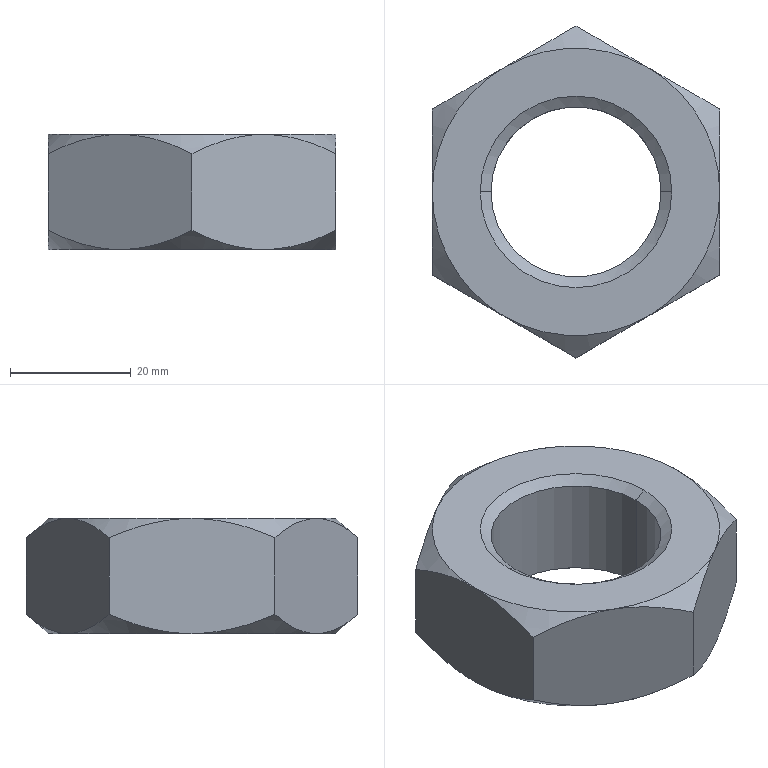Part | SolidWorks | features RevCut 4, Extrusion 1, LPattern 1 | 1 solid | 28 faces | box 47.625 x 54.993 x 19.075 mm | volume 25013 mm3 | cone 16 | plane 8 | cylinder 4 | commonest cylinder face diameters 28.179 x2 31.75 x2
STEP:
#1=CARTESIAN_POINT('',(-0.625,0.,-0.751));
#2=VERTEX_POINT('',#1);
#3=CARTESIAN_POINT('',(0.625,0.,-0.751));
#4=VERTEX_POINT('',#3);
#5=CARTESIAN_POINT('',(0.,0.,-0.751));
#6=DIRECTION('',(0.,0.,1.));
#7=DIRECTION('',(-1.,0.,0.));
#8=AXIS2_PLACEMENT_3D('',#5,#6,#7);
#9=CIRCLE('',#8,0.625);
#10=EDGE_CURVE('',#2,#4,#9,.T.);
#11=ORIENTED_EDGE('',*,*,#10,.F.);
#12=CARTESIAN_POINT('',(-0.625,0.,-0.75));
#13=VERTEX_POINT('',#12);
#14=CARTESIAN_POINT('',(-0.625,0.,-0.9857));
#15=DIRECTION('',(0.,0.,1.));
#16=VECTOR('',#15,39.37);
#17=LINE('',#14,#16);
#18=EDGE_CURVE('',#2,#13,#17,.T.);
#19=ORIENTED_EDGE('',*,*,#18,.T.);
#20=CARTESIAN_POINT('',(0.625,0.,-0.75));
#21=VERTEX_POINT('',#20);
#22=CARTESIAN_POINT('',(0.,0.,-0.75));
#23=DIRECTION('',(0.,0.,1.));
#24=DIRECTION('',(1.,0.,0.));
#25=AXIS2_PLACEMENT_3D('',#22,#23,#24);
#26=CIRCLE('',#25,0.625);
#27=EDGE_CURVE('',#13,#21,#26,.T.);
#28=ORIENTED_EDGE('',*,*,#27,.T.);
#29=CARTESIAN_POINT('',(0.625,0.,-0.9857));
#30=DIRECTION('',(0.,0.,1.));
#31=VECTOR('',#30,39.37);
#32=LINE('',#29,#31);
#33=EDGE_CURVE('',#4,#21,#32,.T.);
#34=ORIENTED_EDGE('',*,*,#33,.F.);
#35=EDGE_LOOP('',(#11,#19,#28,#34));
#36=FACE_OUTER_BOUND('',#35,.T.);
#37=CARTESIAN_POINT('',(0.,0.,-0.9857));
#38=DIRECTION('',(0.,0.,1.));
#39=DIRECTION('',(1.,0.,0.));
#40=AXIS2_PLACEMENT_3D('',#37,#38,#39);
#41=CYLINDRICAL_SURFACE('',#40,0.625);
#42=ADVANCED_FACE('',(#36),#41,.F.);
#43=CARTESIAN_POINT('',(-0.5547,0.,-0.7008));
#44=VERTEX_POINT('',#43);
#45=CARTESIAN_POINT('',(0.5547,0.,-0.7008));
#46=VERTEX_POINT('',#45);
#47=CARTESIAN_POINT('',(0.,0.,-0.7008));
#48=DIRECTION('',(0.,0.,1.));
#49=DIRECTION('',(-1.,0.,0.));
#50=AXIS2_PLACEMENT_3D('',#47,#48,#49);
#51=CIRCLE('',#50,0.5547);
#52=EDGE_CURVE('',#44,#46,#51,.T.);
#53=ORIENTED_EDGE('',*,*,#52,.T.);
#54=CARTESIAN_POINT('',(0.625,0.,-0.75));
#55=DIRECTION('',(0.8192,0.,-0.5736));
#56=VECTOR('',#55,39.37);
#57=LINE('',#54,#56);
#58=EDGE_CURVE('',#46,#21,#57,.T.);
#59=ORIENTED_EDGE('',*,*,#58,.T.);
#60=ORIENTED_EDGE('',*,*,#27,.F.);
#61=CARTESIAN_POINT('',(-0.625,0.,-0.75));
#62=DIRECTION('',(-0.8192,0.,-0.5736));
#63=VECTOR('',#62,39.37);
#64=LINE('',#61,#63);
#65=EDGE_CURVE('',#44,#13,#64,.T.);
#66=ORIENTED_EDGE('',*,*,#65,.F.);
#67=EDGE_LOOP('',(#53,#59,#60,#66));
#68=FACE_OUTER_BOUND('',#67,.T.);
#69=CARTESIAN_POINT('',(0.,0.,-0.75));
#70=DIRECTION('',(0.,0.,-1.));
#71=DIRECTION('',(-1.,0.,0.));
#72=AXIS2_PLACEMENT_3D('',#69,#70,#71);
#73=CONICAL_SURFACE('',#72,0.625,0.9599);
#74=ADVANCED_FACE('',(#68),#73,.F.);
#75=CARTESIAN_POINT('',(0.5547,0.,-0.04922));
#76=VERTEX_POINT('',#75);
#77=CARTESIAN_POINT('',(-0.5547,0.,-0.04922));
#78=VERTEX_POINT('',#77);
#79=CARTESIAN_POINT('',(0.,0.,-0.04922));
#80=DIRECTION('',(0.,0.,-1.));
#81=DIRECTION('',(1.,0.,0.));
#82=AXIS2_PLACEMENT_3D('',#79,#80,#81);
#83=CIRCLE('',#82,0.5547);
#84=EDGE_CURVE('',#76,#78,#83,.T.);
#85=ORIENTED_EDGE('',*,*,#84,.T.);
#86=CARTESIAN_POINT('',(-0.625,0.,0.));
#87=VERTEX_POINT('',#86);
#88=CARTESIAN_POINT('',(-0.5477,0.,-0.05415));
#89=DIRECTION('',(-0.8192,0.,0.5736));
#90=VECTOR('',#89,39.37);
#91=LINE('',#88,#90);
#92=EDGE_CURVE('',#78,#87,#91,.T.);
#93=ORIENTED_EDGE('',*,*,#92,.T.);
#94=CARTESIAN_POINT('',(0.625,0.,0.));
#95=VERTEX_POINT('',#94);
#96=CARTESIAN_POINT('',(0.,0.,0.));
#97=DIRECTION('',(0.,0.,1.));
#98=DIRECTION('',(1.,0.,0.));
#99=AXIS2_PLACEMENT_3D('',#96,#97,#98);
#100=CIRCLE('',#99,0.625);
#101=EDGE_CURVE('',#87,#95,#100,.T.);
#102=ORIENTED_EDGE('',*,*,#101,.T.);
#103=CARTESIAN_POINT('',(0.5477,0.,-0.05415));
#104=DIRECTION('',(0.8192,0.,0.5736));
#105=VECTOR('',#104,39.37);
#106=LINE('',#103,#105);
#107=EDGE_CURVE('',#76,#95,#106,.T.);
#108=ORIENTED_EDGE('',*,*,#107,.F.);
#109=EDGE_LOOP('',(#85,#93,#102,#108));
#110=FACE_OUTER_BOUND('',#109,.T.);
#111=CARTESIAN_POINT('',(0.,0.,-0.05415));
#112=DIRECTION('',(0.,0.,1.));
#113=DIRECTION('',(1.,0.,0.));
#114=AXIS2_PLACEMENT_3D('',#111,#112,#113);
#115=CONICAL_SURFACE('',#114,0.5477,0.9599);
#116=ADVANCED_FACE('',(#110),#115,.F.);
#117=ORIENTED_EDGE('',*,*,#52,.F.);
#118=CARTESIAN_POINT('',(-0.5547,0.,-0.751));
#119=DIRECTION('',(0.,0.,1.));
#120=VECTOR('',#119,39.37);
#121=LINE('',#118,#120);
#122=EDGE_CURVE('',#44,#78,#121,.T.);
#123=ORIENTED_EDGE('',*,*,#122,.T.);
#124=ORIENTED_EDGE('',*,*,#84,.F.);
#125=CARTESIAN_POINT('',(0.5547,0.,-0.751));
#126=DIRECTION('',(0.,0.,1.));
#127=VECTOR('',#126,39.37);
#128=LINE('',#125,#127);
#129=EDGE_CURVE('',#46,#76,#128,.T.);
#130=ORIENTED_EDGE('',*,*,#129,.F.);
#131=EDGE_LOOP('',(#117,#123,#124,#130));
#132=FACE_OUTER_BOUND('',#131,.T.);
#133=CARTESIAN_POINT('',(0.,0.,-0.751));
#134=DIRECTION('',(0.,0.,1.));
#135=DIRECTION('',(1.,0.,0.));
#136=AXIS2_PLACEMENT_3D('',#133,#134,#135);
#137=CYLINDRICAL_SURFACE('',#136,0.5547);
#138=ADVANCED_FACE('',(#132),#137,.F.);
#139=ORIENTED_EDGE('',*,*,#122,.F.);
#140=CARTESIAN_POINT('',(0.,0.,-0.7008));
#141=DIRECTION('',(0.,0.,1.));
#142=DIRECTION('',(-1.,0.,0.));
#143=AXIS2_PLACEMENT_3D('',#140,#141,#142);
#144=CIRCLE('',#143,0.5547);
#145=EDGE_CURVE('',#46,#44,#144,.T.);
#146=ORIENTED_EDGE('',*,*,#145,.F.);
#147=ORIENTED_EDGE('',*,*,#129,.T.);
#148=CARTESIAN_POINT('',(0.,0.,-0.04922));
#149=DIRECTION('',(0.,0.,-1.));
#150=DIRECTION('',(1.,0.,0.));
#151=AXIS2_PLACEMENT_3D('',#148,#149,#150);
#152=CIRCLE('',#151,0.5547);
#153=EDGE_CURVE('',#78,#76,#152,.T.);
#154=ORIENTED_EDGE('',*,*,#153,.F.);
#155=EDGE_LOOP('',(#139,#146,#147,#154));
#156=FACE_OUTER_BOUND('',#155,.T.);
#157=CARTESIAN_POINT('',(0.,0.,-0.751));
#158=DIRECTION('',(0.,0.,1.));
#159=DIRECTION('',(1.,0.,0.));
#160=AXIS2_PLACEMENT_3D('',#157,#158,#159);
#161=CYLINDRICAL_SURFACE('',#160,0.5547);
#162=ADVANCED_FACE('',(#156),#161,.F.);
#163=CARTESIAN_POINT('',(-0.9375,0.5413,-0.626));
#164=VERTEX_POINT('',#163);
#165=CARTESIAN_POINT('',(-0.9375,0.5413,-0.125));
#166=VERTEX_POINT('',#165);
#167=CARTESIAN_POINT('',(-0.9375,0.5413,-0.751));
#168=DIRECTION('',(0.,0.,1.));
#169=VECTOR('',#168,39.37);
#170=LINE('',#167,#169);
#171=EDGE_CURVE('',#164,#166,#170,.T.);
#172=ORIENTED_EDGE('',*,*,#171,.T.);
#173=CARTESIAN_POINT('',(-0.4688,0.8119,0.));
#174=VERTEX_POINT('',#173);
#175=CARTESIAN_POINT('',(-0.9375,0.5413,-0.125));
#176=CARTESIAN_POINT('',(-0.8627,0.5845,-0.08778));
#177=CARTESIAN_POINT('',(-0.7867,0.6283,-0.05655));
#178=CARTESIAN_POINT('',(-0.6698,0.6958,-0.02358));
#179=CARTESIAN_POINT('',(-0.6304,0.7186,-0.01492));
#180=CARTESIAN_POINT('',(-0.5704,0.7532,-0.006076));
#181=CARTESIAN_POINT('',(-0.5503,0.7648,-0.003818));
#182=CARTESIAN_POINT('',(-0.5098,0.7882,-0.0007797));
#183=CARTESIAN_POINT('',(-0.4893,0.8,0.));
#184=CARTESIAN_POINT('',(-0.4688,0.8119,0.));
#185=B_SPLINE_CURVE_WITH_KNOTS('',3,(#175,#176,#177,#178,#179,#180,#181,#182,#183,#184),.UNSPECIFIED.,.F.,.F.,(4,2,2,2,4),(0.000000248,0.007055,0.01058,0.01235,0.01411),.UNSPECIFIED.);
#186=EDGE_CURVE('',#166,#174,#185,.T.);
#187=ORIENTED_EDGE('',*,*,#186,.T.);
#188=CARTESIAN_POINT('',(0.,1.083,-0.125));
#189=VERTEX_POINT('',#188);
#190=CARTESIAN_POINT('',(-0.4688,0.8119,0.));
#191=CARTESIAN_POINT('',(-0.3871,0.8591,0.));
#192=CARTESIAN_POINT('',(-0.3075,0.905,-0.01242));
#193=CARTESIAN_POINT('',(-0.1905,0.9726,-0.04534));
#194=CARTESIAN_POINT('',(-0.1518,0.9949,-0.05867));
#195=CARTESIAN_POINT('',(-0.07528,1.039,-0.08921));
#196=CARTESIAN_POINT('',(-0.03734,1.061,-0.1064));
#197=CARTESIAN_POINT('',(0.,1.083,-0.125));
#198=B_SPLINE_CURVE_WITH_KNOTS('',3,(#190,#191,#192,#193,#194,#195,#196,#197),.UNSPECIFIED.,.F.,.F.,(4,2,2,4),(0.01411,0.02113,0.02464,0.02815),.UNSPECIFIED.);
#199=EDGE_CURVE('',#174,#189,#198,.T.);
#200=ORIENTED_EDGE('',*,*,#199,.T.);
#201=CARTESIAN_POINT('',(0.,1.083,-0.626));
#202=VERTEX_POINT('',#201);
#203=CARTESIAN_POINT('',(0.,1.083,-0.751));
#204=DIRECTION('',(0.,0.,1.));
#205=VECTOR('',#204,39.37);
#206=LINE('',#203,#205);
#207=EDGE_CURVE('',#202,#189,#206,.T.);
#208=ORIENTED_EDGE('',*,*,#207,.F.);
#209=CARTESIAN_POINT('',(-0.4688,0.8119,-0.751));
#210=VERTEX_POINT('',#209);
#211=CARTESIAN_POINT('',(-0.4688,0.8119,-0.751));
#212=CARTESIAN_POINT('',(-0.3871,0.8591,-0.751));
#213=CARTESIAN_POINT('',(-0.3075,0.905,-0.7386));
#214=CARTESIAN_POINT('',(-0.1905,0.9726,-0.7057));
#215=CARTESIAN_POINT('',(-0.1518,0.9949,-0.6923));
#216=CARTESIAN_POINT('',(-0.07528,1.039,-0.6618));
#217=CARTESIAN_POINT('',(-0.03734,1.061,-0.6446));
#218=CARTESIAN_POINT('',(0.,1.083,-0.626));
#219=B_SPLINE_CURVE_WITH_KNOTS('',3,(#211,#212,#213,#214,#215,#216,#217,#218),.UNSPECIFIED.,.F.,.F.,(4,2,2,4),(0.01411,0.02113,0.02464,0.02815),.UNSPECIFIED.);
#220=EDGE_CURVE('',#210,#202,#219,.T.);
#221=ORIENTED_EDGE('',*,*,#220,.F.);
#222=CARTESIAN_POINT('',(-0.9375,0.5413,-0.626));
#223=CARTESIAN_POINT('',(-0.8627,0.5845,-0.6632));
#224=CARTESIAN_POINT('',(-0.7867,0.6283,-0.6944));
#225=CARTESIAN_POINT('',(-0.6698,0.6958,-0.7274));
#226=CARTESIAN_POINT('',(-0.6304,0.7186,-0.7361));
#227=CARTESIAN_POINT('',(-0.5704,0.7532,-0.7449));
#228=CARTESIAN_POINT('',(-0.5503,0.7648,-0.7472));
#229=CARTESIAN_POINT('',(-0.5098,0.7882,-0.7502));
#230=CARTESIAN_POINT('',(-0.4893,0.8,-0.751));
#231=CARTESIAN_POINT('',(-0.4688,0.8119,-0.751));
#232=B_SPLINE_CURVE_WITH_KNOTS('',3,(#222,#223,#224,#225,#226,#227,#228,#229,#230,#231),.UNSPECIFIED.,.F.,.F.,(4,2,2,2,4),(0.000000248,0.007055,0.01058,0.01235,0.01411),.UNSPECIFIED.);
#233=EDGE_CURVE('',#164,#210,#232,.T.);
#234=ORIENTED_EDGE('',*,*,#233,.F.);
#235=EDGE_LOOP('',(#172,#187,#200,#208,#221,#234));
#236=FACE_OUTER_BOUND('',#235,.T.);
#237=CARTESIAN_POINT('',(0.,1.083,-0.751));
#238=DIRECTION('',(-0.5,0.866,0.));
#239=DIRECTION('',(-0.866,-0.5,0.));
#240=AXIS2_PLACEMENT_3D('',#237,#238,#239);
#241=PLANE('',#240);
#242=ADVANCED_FACE('',(#236),#241,.T.);
#243=ORIENTED_EDGE('',*,*,#207,.T.);
#244=CARTESIAN_POINT('',(0.4688,0.8119,0.));
#245=VERTEX_POINT('',#244);
#246=CARTESIAN_POINT('',(0.,1.083,-0.125));
#247=CARTESIAN_POINT('',(0.0748,1.039,-0.08778));
#248=CARTESIAN_POINT('',(0.1508,0.9955,-0.05655));
#249=CARTESIAN_POINT('',(0.2677,0.928,-0.02358));
#250=CARTESIAN_POINT('',(0.3071,0.9052,-0.01492));
#251=CARTESIAN_POINT('',(0.3671,0.8706,-0.006076));
#252=CARTESIAN_POINT('',(0.3872,0.859,-0.003818));
#253=CARTESIAN_POINT('',(0.4277,0.8356,-0.0007797));
#254=CARTESIAN_POINT('',(0.4482,0.8237,0.));
#255=CARTESIAN_POINT('',(0.4688,0.8119,0.));
#256=B_SPLINE_CURVE_WITH_KNOTS('',3,(#246,#247,#248,#249,#250,#251,#252,#253,#254,#255),.UNSPECIFIED.,.F.,.F.,(4,2,2,2,4),(0.000000248,0.007055,0.01058,0.01235,0.01411),.UNSPECIFIED.);
#257=EDGE_CURVE('',#189,#245,#256,.T.);
#258=ORIENTED_EDGE('',*,*,#257,.T.);
#259=CARTESIAN_POINT('',(0.9375,0.5413,-0.125));
#260=VERTEX_POINT('',#259);
#261=CARTESIAN_POINT('',(0.4688,0.8119,0.));
#262=CARTESIAN_POINT('',(0.5504,0.7647,0.));
#263=CARTESIAN_POINT('',(0.63,0.7188,-0.01242));
#264=CARTESIAN_POINT('',(0.747,0.6512,-0.04534));
#265=CARTESIAN_POINT('',(0.7857,0.6289,-0.05867));
#266=CARTESIAN_POINT('',(0.8622,0.5847,-0.08921));
#267=CARTESIAN_POINT('',(0.9002,0.5628,-0.1064));
#268=CARTESIAN_POINT('',(0.9375,0.5413,-0.125));
#269=B_SPLINE_CURVE_WITH_KNOTS('',3,(#261,#262,#263,#264,#265,#266,#267,#268),.UNSPECIFIED.,.F.,.F.,(4,2,2,4),(0.01411,0.02113,0.02464,0.02815),.UNSPECIFIED.);
#270=EDGE_CURVE('',#245,#260,#269,.T.);
#271=ORIENTED_EDGE('',*,*,#270,.T.);
#272=CARTESIAN_POINT('',(0.9375,0.5413,-0.626));
#273=VERTEX_POINT('',#272);
#274=CARTESIAN_POINT('',(0.9375,0.5413,-0.751));
#275=DIRECTION('',(0.,0.,1.));
#276=VECTOR('',#275,39.37);
#277=LINE('',#274,#276);
#278=EDGE_CURVE('',#273,#260,#277,.T.);
#279=ORIENTED_EDGE('',*,*,#278,.F.);
#280=CARTESIAN_POINT('',(0.4688,0.8119,-0.751));
#281=VERTEX_POINT('',#280);
#282=CARTESIAN_POINT('',(0.4688,0.8119,-0.751));
#283=CARTESIAN_POINT('',(0.5504,0.7647,-0.751));
#284=CARTESIAN_POINT('',(0.63,0.7188,-0.7386));
#285=CARTESIAN_POINT('',(0.747,0.6512,-0.7057));
#286=CARTESIAN_POINT('',(0.7857,0.6289,-0.6923));
#287=CARTESIAN_POINT('',(0.8622,0.5847,-0.6618));
#288=CARTESIAN_POINT('',(0.9002,0.5628,-0.6446));
#289=CARTESIAN_POINT('',(0.9375,0.5413,-0.626));
#290=B_SPLINE_CURVE_WITH_KNOTS('',3,(#282,#283,#284,#285,#286,#287,#288,#289),.UNSPECIFIED.,.F.,.F.,(4,2,2,4),(0.01411,0.02113,0.02464,0.02815),.UNSPECIFIED.);
#291=EDGE_CURVE('',#281,#273,#290,.T.);
#292=ORIENTED_EDGE('',*,*,#291,.F.);
#293=CARTESIAN_POINT('',(0.,1.083,-0.626));
#294=CARTESIAN_POINT('',(0.0748,1.039,-0.6632));
#295=CARTESIAN_POINT('',(0.1508,0.9955,-0.6944));
#296=CARTESIAN_POINT('',(0.2677,0.928,-0.7274));
#297=CARTESIAN_POINT('',(0.3071,0.9052,-0.7361));
#298=CARTESIAN_POINT('',(0.3671,0.8706,-0.7449));
#299=CARTESIAN_POINT('',(0.3872,0.859,-0.7472));
#300=CARTESIAN_POINT('',(0.4277,0.8356,-0.7502));
#301=CARTESIAN_POINT('',(0.4482,0.8237,-0.751));
#302=CARTESIAN_POINT('',(0.4688,0.8119,-0.751));
#303=B_SPLINE_CURVE_WITH_KNOTS('',3,(#293,#294,#295,#296,#297,#298,#299,#300,#301,#302),.UNSPECIFIED.,.F.,.F.,(4,2,2,2,4),(0.000000248,0.007055,0.01058,0.01235,0.01411),.UNSPECIFIED.);
#304=EDGE_CURVE('',#202,#281,#303,.T.);
#305=ORIENTED_EDGE('',*,*,#304,.F.);
#306=EDGE_LOOP('',(#243,#258,#271,#279,#292,#305));
#307=FACE_OUTER_BOUND('',#306,.T.);
#308=CARTESIAN_POINT('',(0.9375,0.5413,-0.751));
#309=DIRECTION('',(0.5,0.866,0.));
#310=DIRECTION('',(-0.866,0.5,0.));
#311=AXIS2_PLACEMENT_3D('',#308,#309,#310);
#312=PLANE('',#311);
#313=ADVANCED_FACE('',(#307),#312,.T.);
#314=CARTESIAN_POINT('',(0.9375,-0.5413,-0.125));
#315=VERTEX_POINT('',#314);
#316=CARTESIAN_POINT('',(0.9375,0.,0.));
#317=VERTEX_POINT('',#316);
#318=CARTESIAN_POINT('',(0.9375,-0.5413,-0.125));
#319=CARTESIAN_POINT('',(0.9375,-0.4985,-0.1066));
#320=CARTESIAN_POINT('',(0.9375,-0.4551,-0.08948));
#321=CARTESIAN_POINT('',(0.9375,-0.3663,-0.05876));
#322=CARTESIAN_POINT('',(0.9375,-0.3214,-0.04534));
#323=CARTESIAN_POINT('',(0.9375,-0.1858,-0.01233));
#324=CARTESIAN_POINT('',(0.9375,-0.09391,0.));
#325=CARTESIAN_POINT('',(0.9375,0.,0.));
#326=B_SPLINE_CURVE_WITH_KNOTS('',3,(#318,#319,#320,#321,#322,#323,#324,#325),.UNSPECIFIED.,.F.,.F.,(4,2,2,4),(0.01925,0.02278,0.02631,0.03337),.UNSPECIFIED.);
#327=EDGE_CURVE('',#315,#317,#326,.T.);
#328=ORIENTED_EDGE('',*,*,#327,.F.);
#329=CARTESIAN_POINT('',(0.9375,-0.5413,-0.626));
#330=VERTEX_POINT('',#329);
#331=CARTESIAN_POINT('',(0.9375,-0.5413,-0.751));
#332=DIRECTION('',(0.,0.,1.));
#333=VECTOR('',#332,39.37);
#334=LINE('',#331,#333);
#335=EDGE_CURVE('',#330,#315,#334,.T.);
#336=ORIENTED_EDGE('',*,*,#335,.F.);
#337=CARTESIAN_POINT('',(0.9375,0.,-0.751));
#338=VERTEX_POINT('',#337);
#339=CARTESIAN_POINT('',(0.9375,-0.5413,-0.626));
#340=CARTESIAN_POINT('',(0.9375,-0.4985,-0.6444));
#341=CARTESIAN_POINT('',(0.9375,-0.4551,-0.6615));
#342=CARTESIAN_POINT('',(0.9375,-0.3663,-0.6922));
#343=CARTESIAN_POINT('',(0.9375,-0.3214,-0.7057));
#344=CARTESIAN_POINT('',(0.9375,-0.1858,-0.7387));
#345=CARTESIAN_POINT('',(0.9375,-0.09391,-0.751));
#346=CARTESIAN_POINT('',(0.9375,0.,-0.751));
#347=B_SPLINE_CURVE_WITH_KNOTS('',3,(#339,#340,#341,#342,#343,#344,#345,#346),.UNSPECIFIED.,.F.,.F.,(4,2,2,4),(0.01925,0.02278,0.02631,0.03337),.UNSPECIFIED.);
#348=EDGE_CURVE('',#330,#338,#347,.T.);
#349=ORIENTED_EDGE('',*,*,#348,.T.);
#350=CARTESIAN_POINT('',(0.9375,0.,-0.751));
#351=CARTESIAN_POINT('',(0.9375,0.0234,-0.751));
#352=CARTESIAN_POINT('',(0.9375,0.047,-0.7502));
#353=CARTESIAN_POINT('',(0.9375,0.09377,-0.7472));
#354=CARTESIAN_POINT('',(0.9375,0.117,-0.745));
#355=CARTESIAN_POINT('',(0.9375,0.1862,-0.7362));
#356=CARTESIAN_POINT('',(0.9375,0.2318,-0.7275));
#357=CARTESIAN_POINT('',(0.9375,0.322,-0.7055));
#358=CARTESIAN_POINT('',(0.9375,0.3666,-0.6921));
#359=CARTESIAN_POINT('',(0.9375,0.4329,-0.6692));
#360=CARTESIAN_POINT('',(0.9375,0.4549,-0.6611));
#361=CARTESIAN_POINT('',(0.9375,0.4984,-0.6441));
#362=CARTESIAN_POINT('',(0.9375,0.5199,-0.6352));
#363=CARTESIAN_POINT('',(0.9375,0.5413,-0.626));
#364=B_SPLINE_CURVE_WITH_KNOTS('',3,(#350,#351,#352,#353,#354,#355,#356,#357,#358,#359,#360,#361,#362,#363),.UNSPECIFIED.,.F.,.F.,(4,2,2,2,2,2,4),(0.03337,0.03513,0.03689,0.04041,0.04394,0.0457,0.04746),.UNSPECIFIED.);
#365=EDGE_CURVE('',#338,#273,#364,.T.);
#366=ORIENTED_EDGE('',*,*,#365,.T.);
#367=ORIENTED_EDGE('',*,*,#278,.T.);
#368=CARTESIAN_POINT('',(0.9375,0.,0.));
#369=CARTESIAN_POINT('',(0.9375,0.0234,0.));
#370=CARTESIAN_POINT('',(0.9375,0.047,-0.0007652));
#371=CARTESIAN_POINT('',(0.9375,0.09377,-0.003783));
#372=CARTESIAN_POINT('',(0.9375,0.117,-0.00603));
#373=CARTESIAN_POINT('',(0.9375,0.1862,-0.01485));
#374=CARTESIAN_POINT('',(0.9375,0.2318,-0.0235));
#375=CARTESIAN_POINT('',(0.9375,0.322,-0.04552));
#376=CARTESIAN_POINT('',(0.9375,0.3666,-0.05887));
#377=CARTESIAN_POINT('',(0.9375,0.4329,-0.0818));
#378=CARTESIAN_POINT('',(0.9375,0.4549,-0.08994));
#379=CARTESIAN_POINT('',(0.9375,0.4984,-0.1069));
#380=CARTESIAN_POINT('',(0.9375,0.5199,-0.1158));
#381=CARTESIAN_POINT('',(0.9375,0.5413,-0.125));
#382=B_SPLINE_CURVE_WITH_KNOTS('',3,(#368,#369,#370,#371,#372,#373,#374,#375,#376,#377,#378,#379,#380,#381),.UNSPECIFIED.,.F.,.F.,(4,2,2,2,2,2,4),(0.03337,0.03513,0.03689,0.04041,0.04394,0.0457,0.04746),.UNSPECIFIED.);
#383=EDGE_CURVE('',#317,#260,#382,.T.);
#384=ORIENTED_EDGE('',*,*,#383,.F.);
#385=EDGE_LOOP('',(#328,#336,#349,#366,#367,#384));
#386=FACE_OUTER_BOUND('',#385,.T.);
#387=CARTESIAN_POINT('',(0.9375,0.5413,-0.751));
#388=DIRECTION('',(-1.,0.,0.));
#389=DIRECTION('',(0.,0.,1.));
#390=AXIS2_PLACEMENT_3D('',#387,#388,#389);
#391=PLANE('',#390);
#392=ADVANCED_FACE('',(#386),#391,.F.);
#393=ORIENTED_EDGE('',*,*,#335,.T.);
#394=CARTESIAN_POINT('',(0.4688,-0.8119,0.));
#395=VERTEX_POINT('',#394);
#396=CARTESIAN_POINT('',(0.9375,-0.5413,-0.125));
#397=CARTESIAN_POINT('',(0.8627,-0.5845,-0.08778));
#398=CARTESIAN_POINT('',(0.7867,-0.6283,-0.05655));
#399=CARTESIAN_POINT('',(0.6698,-0.6958,-0.02358));
#400=CARTESIAN_POINT('',(0.6304,-0.7186,-0.01492));
#401=CARTESIAN_POINT('',(0.5704,-0.7532,-0.006076));
#402=CARTESIAN_POINT('',(0.5503,-0.7648,-0.003818));
#403=CARTESIAN_POINT('',(0.5098,-0.7882,-0.0007797));
#404=CARTESIAN_POINT('',(0.4893,-0.8,0.));
#405=CARTESIAN_POINT('',(0.4688,-0.8119,0.));
#406=B_SPLINE_CURVE_WITH_KNOTS('',3,(#396,#397,#398,#399,#400,#401,#402,#403,#404,#405),.UNSPECIFIED.,.F.,.F.,(4,2,2,2,4),(0.000000248,0.007055,0.01058,0.01235,0.01411),.UNSPECIFIED.);
#407=EDGE_CURVE('',#315,#395,#406,.T.);
#408=ORIENTED_EDGE('',*,*,#407,.T.);
#409=CARTESIAN_POINT('',(0.,-1.083,-0.125));
#410=VERTEX_POINT('',#409);
#411=CARTESIAN_POINT('',(0.4688,-0.8119,0.));
#412=CARTESIAN_POINT('',(0.3871,-0.8591,0.));
#413=CARTESIAN_POINT('',(0.3075,-0.905,-0.01242));
#414=CARTESIAN_POINT('',(0.1905,-0.9726,-0.04534));
#415=CARTESIAN_POINT('',(0.1518,-0.9949,-0.05867));
#416=CARTESIAN_POINT('',(0.07528,-1.039,-0.08921));
#417=CARTESIAN_POINT('',(0.03734,-1.061,-0.1064));
#418=CARTESIAN_POINT('',(0.,-1.083,-0.125));
#419=B_SPLINE_CURVE_WITH_KNOTS('',3,(#411,#412,#413,#414,#415,#416,#417,#418),.UNSPECIFIED.,.F.,.F.,(4,2,2,4),(0.01411,0.02113,0.02464,0.02815),.UNSPECIFIED.);
#420=EDGE_CURVE('',#395,#410,#419,.T.);
#421=ORIENTED_EDGE('',*,*,#420,.T.);
#422=CARTESIAN_POINT('',(0.,-1.083,-0.626));
#423=VERTEX_POINT('',#422);
#424=CARTESIAN_POINT('',(0.,-1.083,-0.751));
#425=DIRECTION('',(0.,0.,1.));
#426=VECTOR('',#425,39.37);
#427=LINE('',#424,#426);
#428=EDGE_CURVE('',#423,#410,#427,.T.);
#429=ORIENTED_EDGE('',*,*,#428,.F.);
#430=CARTESIAN_POINT('',(0.4688,-0.8119,-0.751));
#431=VERTEX_POINT('',#430);
#432=CARTESIAN_POINT('',(0.4688,-0.8119,-0.751));
#433=CARTESIAN_POINT('',(0.3871,-0.8591,-0.751));
#434=CARTESIAN_POINT('',(0.3075,-0.905,-0.7386));
#435=CARTESIAN_POINT('',(0.1905,-0.9726,-0.7057));
#436=CARTESIAN_POINT('',(0.1518,-0.9949,-0.6923));
#437=CARTESIAN_POINT('',(0.07528,-1.039,-0.6618));
#438=CARTESIAN_POINT('',(0.03734,-1.061,-0.6446));
#439=CARTESIAN_POINT('',(0.,-1.083,-0.626));
#440=B_SPLINE_CURVE_WITH_KNOTS('',3,(#432,#433,#434,#435,#436,#437,#438,#439),.UNSPECIFIED.,.F.,.F.,(4,2,2,4),(0.01411,0.02113,0.02464,0.02815),.UNSPECIFIED.);
#441=EDGE_CURVE('',#431,#423,#440,.T.);
#442=ORIENTED_EDGE('',*,*,#441,.F.);
#443=CARTESIAN_POINT('',(0.9375,-0.5413,-0.626));
#444=CARTESIAN_POINT('',(0.8627,-0.5845,-0.6632));
#445=CARTESIAN_POINT('',(0.7867,-0.6283,-0.6944));
#446=CARTESIAN_POINT('',(0.6698,-0.6958,-0.7274));
#447=CARTESIAN_POINT('',(0.6304,-0.7186,-0.7361));
#448=CARTESIAN_POINT('',(0.5704,-0.7532,-0.7449));
#449=CARTESIAN_POINT('',(0.5503,-0.7648,-0.7472));
#450=CARTESIAN_POINT('',(0.5098,-0.7882,-0.7502));
#451=CARTESIAN_POINT('',(0.4893,-0.8,-0.751));
#452=CARTESIAN_POINT('',(0.4688,-0.8119,-0.751));
#453=B_SPLINE_CURVE_WITH_KNOTS('',3,(#443,#444,#445,#446,#447,#448,#449,#450,#451,#452),.UNSPECIFIED.,.F.,.F.,(4,2,2,2,4),(0.000000248,0.007055,0.01058,0.01235,0.01411),.UNSPECIFIED.);
#454=EDGE_CURVE('',#330,#431,#453,.T.);
#455=ORIENTED_EDGE('',*,*,#454,.F.);
#456=EDGE_LOOP('',(#393,#408,#421,#429,#442,#455));
#457=FACE_OUTER_BOUND('',#456,.T.);
#458=CARTESIAN_POINT('',(0.,-1.083,-0.751));
#459=DIRECTION('',(0.5,-0.866,0.));
#460=DIRECTION('',(0.866,0.5,0.));
#461=AXIS2_PLACEMENT_3D('',#458,#459,#460);
#462=PLANE('',#461);
#463=ADVANCED_FACE('',(#457),#462,.T.);
#464=ORIENTED_EDGE('',*,*,#428,.T.);
#465=CARTESIAN_POINT('',(-0.4688,-0.8119,0.));
#466=VERTEX_POINT('',#465);
#467=CARTESIAN_POINT('',(0.,-1.083,-0.125));
#468=CARTESIAN_POINT('',(-0.0748,-1.039,-0.08778));
#469=CARTESIAN_POINT('',(-0.1508,-0.9955,-0.05655));
#470=CARTESIAN_POINT('',(-0.2677,-0.928,-0.02358));
#471=CARTESIAN_POINT('',(-0.3071,-0.9052,-0.01492));
#472=CARTESIAN_POINT('',(-0.3671,-0.8706,-0.006076));
#473=CARTESIAN_POINT('',(-0.3872,-0.859,-0.003818));
#474=CARTESIAN_POINT('',(-0.4277,-0.8356,-0.0007797));
#475=CARTESIAN_POINT('',(-0.4482,-0.8237,0.));
#476=CARTESIAN_POINT('',(-0.4688,-0.8119,0.));
#477=B_SPLINE_CURVE_WITH_KNOTS('',3,(#467,#468,#469,#470,#471,#472,#473,#474,#475,#476),.UNSPECIFIED.,.F.,.F.,(4,2,2,2,4),(0.000000248,0.007055,0.01058,0.01235,0.01411),.UNSPECIFIED.);
#478=EDGE_CURVE('',#410,#466,#477,.T.);
#479=ORIENTED_EDGE('',*,*,#478,.T.);
#480=CARTESIAN_POINT('',(-0.9375,-0.5413,-0.125));
#481=VERTEX_POINT('',#480);
#482=CARTESIAN_POINT('',(-0.4688,-0.8119,0.));
#483=CARTESIAN_POINT('',(-0.5504,-0.7647,0.));
#484=CARTESIAN_POINT('',(-0.63,-0.7188,-0.01242));
#485=CARTESIAN_POINT('',(-0.747,-0.6512,-0.04534));
#486=CARTESIAN_POINT('',(-0.7857,-0.6289,-0.05867));
#487=CARTESIAN_POINT('',(-0.8622,-0.5847,-0.08921));
#488=CARTESIAN_POINT('',(-0.9002,-0.5628,-0.1064));
#489=CARTESIAN_POINT('',(-0.9375,-0.5413,-0.125));
#490=B_SPLINE_CURVE_WITH_KNOTS('',3,(#482,#483,#484,#485,#486,#487,#488,#489),.UNSPECIFIED.,.F.,.F.,(4,2,2,4),(0.01411,0.02113,0.02464,0.02815),.UNSPECIFIED.);
#491=EDGE_CURVE('',#466,#481,#490,.T.);
#492=ORIENTED_EDGE('',*,*,#491,.T.);
#493=CARTESIAN_POINT('',(-0.9375,-0.5413,-0.626));
#494=VERTEX_POINT('',#493);
#495=CARTESIAN_POINT('',(-0.9375,-0.5413,-0.751));
#496=DIRECTION('',(0.,0.,1.));
#497=VECTOR('',#496,39.37);
#498=LINE('',#495,#497);
#499=EDGE_CURVE('',#494,#481,#498,.T.);
#500=ORIENTED_EDGE('',*,*,#499,.F.);
#501=CARTESIAN_POINT('',(-0.4688,-0.8119,-0.751));
#502=VERTEX_POINT('',#501);
#503=CARTESIAN_POINT('',(-0.4688,-0.8119,-0.751));
#504=CARTESIAN_POINT('',(-0.5504,-0.7647,-0.751));
#505=CARTESIAN_POINT('',(-0.63,-0.7188,-0.7386));
#506=CARTESIAN_POINT('',(-0.747,-0.6512,-0.7057));
#507=CARTESIAN_POINT('',(-0.7857,-0.6289,-0.6923));
#508=CARTESIAN_POINT('',(-0.8622,-0.5847,-0.6618));
#509=CARTESIAN_POINT('',(-0.9002,-0.5628,-0.6446));
#510=CARTESIAN_POINT('',(-0.9375,-0.5413,-0.626));
#511=B_SPLINE_CURVE_WITH_KNOTS('',3,(#503,#504,#505,#506,#507,#508,#509,#510),.UNSPECIFIED.,.F.,.F.,(4,2,2,4),(0.01411,0.02113,0.02464,0.02815),.UNSPECIFIED.);
#512=EDGE_CURVE('',#502,#494,#511,.T.);
#513=ORIENTED_EDGE('',*,*,#512,.F.);
#514=CARTESIAN_POINT('',(0.,-1.083,-0.626));
#515=CARTESIAN_POINT('',(-0.0748,-1.039,-0.6632));
#516=CARTESIAN_POINT('',(-0.1508,-0.9955,-0.6944));
#517=CARTESIAN_POINT('',(-0.2677,-0.928,-0.7274));
#518=CARTESIAN_POINT('',(-0.3071,-0.9052,-0.7361));
#519=CARTESIAN_POINT('',(-0.3671,-0.8706,-0.7449));
#520=CARTESIAN_POINT('',(-0.3872,-0.859,-0.7472));
#521=CARTESIAN_POINT('',(-0.4277,-0.8356,-0.7502));
#522=CARTESIAN_POINT('',(-0.4482,-0.8237,-0.751));
#523=CARTESIAN_POINT('',(-0.4688,-0.8119,-0.751));
#524=B_SPLINE_CURVE_WITH_KNOTS('',3,(#514,#515,#516,#517,#518,#519,#520,#521,#522,#523),.UNSPECIFIED.,.F.,.F.,(4,2,2,2,4),(0.000000248,0.007055,0.01058,0.01235,0.01411),.UNSPECIFIED.);
#525=EDGE_CURVE('',#423,#502,#524,.T.);
#526=ORIENTED_EDGE('',*,*,#525,.F.);
#527=EDGE_LOOP('',(#464,#479,#492,#500,#513,#526));
#528=FACE_OUTER_BOUND('',#527,.T.);
#529=CARTESIAN_POINT('',(-0.9375,-0.5413,-0.751));
#530=DIRECTION('',(-0.5,-0.866,0.));
#531=DIRECTION('',(0.866,-0.5,0.));
#532=AXIS2_PLACEMENT_3D('',#529,#530,#531);
#533=PLANE('',#532);
#534=ADVANCED_FACE('',(#528),#533,.T.);
#535=ORIENTED_EDGE('',*,*,#499,.T.);
#536=CARTESIAN_POINT('',(-0.9375,0.,0.));
#537=VERTEX_POINT('',#536);
#538=CARTESIAN_POINT('',(-0.9375,-0.5413,-0.125));
#539=CARTESIAN_POINT('',(-0.9375,-0.4985,-0.1066));
#540=CARTESIAN_POINT('',(-0.9375,-0.4551,-0.08948));
#541=CARTESIAN_POINT('',(-0.9375,-0.3663,-0.05876));
#542=CARTESIAN_POINT('',(-0.9375,-0.3214,-0.04534));
#543=CARTESIAN_POINT('',(-0.9375,-0.1858,-0.01233));
#544=CARTESIAN_POINT('',(-0.9375,-0.09391,0.));
#545=CARTESIAN_POINT('',(-0.9375,0.,0.));
#546=B_SPLINE_CURVE_WITH_KNOTS('',3,(#538,#539,#540,#541,#542,#543,#544,#545),.UNSPECIFIED.,.F.,.F.,(4,2,2,4),(0.01925,0.02278,0.02631,0.03337),.UNSPECIFIED.);
#547=EDGE_CURVE('',#481,#537,#546,.T.);
#548=ORIENTED_EDGE('',*,*,#547,.T.);
#549=CARTESIAN_POINT('',(-0.9375,0.,0.));
#550=CARTESIAN_POINT('',(-0.9375,0.0234,0.));
#551=CARTESIAN_POINT('',(-0.9375,0.047,-0.0007652));
#552=CARTESIAN_POINT('',(-0.9375,0.09377,-0.003783));
#553=CARTESIAN_POINT('',(-0.9375,0.117,-0.00603));
#554=CARTESIAN_POINT('',(-0.9375,0.1862,-0.01485));
#555=CARTESIAN_POINT('',(-0.9375,0.2318,-0.0235));
#556=CARTESIAN_POINT('',(-0.9375,0.322,-0.04552));
#557=CARTESIAN_POINT('',(-0.9375,0.3666,-0.05887));
#558=CARTESIAN_POINT('',(-0.9375,0.4329,-0.0818));
#559=CARTESIAN_POINT('',(-0.9375,0.4549,-0.08994));
#560=CARTESIAN_POINT('',(-0.9375,0.4984,-0.1069));
#561=CARTESIAN_POINT('',(-0.9375,0.5199,-0.1158));
#562=CARTESIAN_POINT('',(-0.9375,0.5413,-0.125));
#563=B_SPLINE_CURVE_WITH_KNOTS('',3,(#549,#550,#551,#552,#553,#554,#555,#556,#557,#558,#559,#560,#561,#562),.UNSPECIFIED.,.F.,.F.,(4,2,2,2,2,2,4),(0.03337,0.03513,0.03689,0.04041,0.04394,0.0457,0.04746),.UNSPECIFIED.);
#564=EDGE_CURVE('',#537,#166,#563,.T.);
#565=ORIENTED_EDGE('',*,*,#564,.T.);
#566=ORIENTED_EDGE('',*,*,#171,.F.);
#567=CARTESIAN_POINT('',(-0.9375,0.,-0.751));
#568=VERTEX_POINT('',#567);
#569=CARTESIAN_POINT('',(-0.9375,0.,-0.751));
#570=CARTESIAN_POINT('',(-0.9375,0.0234,-0.751));
#571=CARTESIAN_POINT('',(-0.9375,0.047,-0.7502));
#572=CARTESIAN_POINT('',(-0.9375,0.09377,-0.7472));
#573=CARTESIAN_POINT('',(-0.9375,0.117,-0.745));
#574=CARTESIAN_POINT('',(-0.9375,0.1862,-0.7362));
#575=CARTESIAN_POINT('',(-0.9375,0.2318,-0.7275));
#576=CARTESIAN_POINT('',(-0.9375,0.322,-0.7055));
#577=CARTESIAN_POINT('',(-0.9375,0.3666,-0.6921));
#578=CARTESIAN_POINT('',(-0.9375,0.4329,-0.6692));
#579=CARTESIAN_POINT('',(-0.9375,0.4549,-0.6611));
#580=CARTESIAN_POINT('',(-0.9375,0.4984,-0.6441));
#581=CARTESIAN_POINT('',(-0.9375,0.5199,-0.6352));
#582=CARTESIAN_POINT('',(-0.9375,0.5413,-0.626));
#583=B_SPLINE_CURVE_WITH_KNOTS('',3,(#569,#570,#571,#572,#573,#574,#575,#576,#577,#578,#579,#580,#581,#582),.UNSPECIFIED.,.F.,.F.,(4,2,2,2,2,2,4),(0.03337,0.03513,0.03689,0.04041,0.04394,0.0457,0.04746),.UNSPECIFIED.);
#584=EDGE_CURVE('',#568,#164,#583,.T.);
#585=ORIENTED_EDGE('',*,*,#584,.F.);
#586=CARTESIAN_POINT('',(-0.9375,-0.5413,-0.626));
#587=CARTESIAN_POINT('',(-0.9375,-0.4985,-0.6444));
#588=CARTESIAN_POINT('',(-0.9375,-0.4551,-0.6615));
#589=CARTESIAN_POINT('',(-0.9375,-0.3663,-0.6922));
#590=CARTESIAN_POINT('',(-0.9375,-0.3214,-0.7057));
#591=CARTESIAN_POINT('',(-0.9375,-0.1858,-0.7387));
#592=CARTESIAN_POINT('',(-0.9375,-0.09391,-0.751));
#593=CARTESIAN_POINT('',(-0.9375,0.,-0.751));
#594=B_SPLINE_CURVE_WITH_KNOTS('',3,(#586,#587,#588,#589,#590,#591,#592,#593),.UNSPECIFIED.,.F.,.F.,(4,2,2,4),(0.01925,0.02278,0.02631,0.03337),.UNSPECIFIED.);
#595=EDGE_CURVE('',#494,#568,#594,.T.);
#596=ORIENTED_EDGE('',*,*,#595,.F.);
#597=EDGE_LOOP('',(#535,#548,#565,#566,#585,#596));
#598=FACE_OUTER_BOUND('',#597,.T.);
#599=CARTESIAN_POINT('',(-0.9375,0.5413,-0.751));
#600=DIRECTION('',(-1.,0.,0.));
#601=DIRECTION('',(0.,0.,1.));
#602=AXIS2_PLACEMENT_3D('',#599,#600,#601);
#603=PLANE('',#602);
#604=ADVANCED_FACE('',(#598),#603,.T.);
#605=CARTESIAN_POINT('',(0.,0.,0.));
#606=DIRECTION('',(0.,0.,1.));
#607=DIRECTION('',(1.,0.,0.));
#608=AXIS2_PLACEMENT_3D('',#605,#606,#607);
#609=CIRCLE('',#608,0.625);
#610=EDGE_CURVE('',#95,#87,#609,.T.);
#611=ORIENTED_EDGE('',*,*,#610,.F.);
#612=ORIENTED_EDGE('',*,*,#101,.F.);
#613=EDGE_LOOP('',(#611,#612));
#614=FACE_BOUND('',#613,.T.);
#615=CARTESIAN_POINT('',(0.,0.,0.));
#616=DIRECTION('',(0.,0.,-1.));
#617=DIRECTION('',(-1.,0.,0.));
#618=AXIS2_PLACEMENT_3D('',#615,#616,#617);
#619=CIRCLE('',#618,0.9375);
#620=EDGE_CURVE('',#537,#174,#619,.T.);
#621=ORIENTED_EDGE('',*,*,#620,.F.);
#622=CARTESIAN_POINT('',(0.,0.,0.));
#623=DIRECTION('',(0.,0.,-1.));
#624=DIRECTION('',(-1.,0.,0.));
#625=AXIS2_PLACEMENT_3D('',#622,#623,#624);
#626=CIRCLE('',#625,0.9375);
#627=EDGE_CURVE('',#466,#537,#626,.T.);
#628=ORIENTED_EDGE('',*,*,#627,.F.);
#629=CARTESIAN_POINT('',(0.,0.,0.));
#630=DIRECTION('',(0.,0.,-1.));
#631=DIRECTION('',(-1.,0.,0.));
#632=AXIS2_PLACEMENT_3D('',#629,#630,#631);
#633=CIRCLE('',#632,0.9375);
#634=EDGE_CURVE('',#395,#466,#633,.T.);
#635=ORIENTED_EDGE('',*,*,#634,.F.);
#636=CARTESIAN_POINT('',(0.,0.,0.));
#637=DIRECTION('',(0.,0.,-1.));
#638=DIRECTION('',(-1.,0.,0.));
#639=AXIS2_PLACEMENT_3D('',#636,#637,#638);
#640=CIRCLE('',#639,0.9375);
#641=EDGE_CURVE('',#317,#395,#640,.T.);
#642=ORIENTED_EDGE('',*,*,#641,.F.);
#643=CARTESIAN_POINT('',(0.,0.,0.));
#644=DIRECTION('',(0.,0.,1.));
#645=DIRECTION('',(1.,0.,0.));
#646=AXIS2_PLACEMENT_3D('',#643,#644,#645);
#647=CIRCLE('',#646,0.9375);
#648=EDGE_CURVE('',#317,#245,#647,.T.);
#649=ORIENTED_EDGE('',*,*,#648,.T.);
#650=CARTESIAN_POINT('',(0.,0.,0.));
#651=DIRECTION('',(0.,0.,-1.));
#652=DIRECTION('',(-1.,0.,0.));
#653=AXIS2_PLACEMENT_3D('',#650,#651,#652);
#654=CIRCLE('',#653,0.9375);
#655=EDGE_CURVE('',#174,#245,#654,.T.);
#656=ORIENTED_EDGE('',*,*,#655,.F.);
#657=EDGE_LOOP('',(#621,#628,#635,#642,#649,#656));
#658=FACE_OUTER_BOUND('',#657,.T.);
#659=CARTESIAN_POINT('',(0.,1.083,0.));
#660=DIRECTION('',(0.,0.,-1.));
#661=DIRECTION('',(-1.,0.,0.));
#662=AXIS2_PLACEMENT_3D('',#659,#660,#661);
#663=PLANE('',#662);
#664=ADVANCED_FACE('',(#614,#658),#663,.F.);
#665=CARTESIAN_POINT('',(0.,0.,-0.751));
#666=DIRECTION('',(0.,0.,1.));
#667=DIRECTION('',(-1.,0.,0.));
#668=AXIS2_PLACEMENT_3D('',#665,#666,#667);
#669=CIRCLE('',#668,0.625);
#670=EDGE_CURVE('',#4,#2,#669,.T.);
#671=ORIENTED_EDGE('',*,*,#670,.T.);
#672=ORIENTED_EDGE('',*,*,#10,.T.);
#673=EDGE_LOOP('',(#671,#672));
#674=FACE_BOUND('',#673,.T.);
#675=CARTESIAN_POINT('',(0.,0.,-0.751));
#676=DIRECTION('',(0.,0.,1.));
#677=DIRECTION('',(-1.,0.,0.));
#678=AXIS2_PLACEMENT_3D('',#675,#676,#677);
#679=CIRCLE('',#678,0.9375);
#680=EDGE_CURVE('',#568,#502,#679,.T.);
#681=ORIENTED_EDGE('',*,*,#680,.F.);
#682=CARTESIAN_POINT('',(0.,0.,-0.751));
#683=DIRECTION('',(0.,0.,1.));
#684=DIRECTION('',(-1.,0.,0.));
#685=AXIS2_PLACEMENT_3D('',#682,#683,#684);
#686=CIRCLE('',#685,0.9375);
#687=EDGE_CURVE('',#210,#568,#686,.T.);
#688=ORIENTED_EDGE('',*,*,#687,.F.);
#689=CARTESIAN_POINT('',(0.,0.,-0.751));
#690=DIRECTION('',(0.,0.,1.));
#691=DIRECTION('',(-1.,0.,0.));
#692=AXIS2_PLACEMENT_3D('',#689,#690,#691);
#693=CIRCLE('',#692,0.9375);
#694=EDGE_CURVE('',#281,#210,#693,.T.);
#695=ORIENTED_EDGE('',*,*,#694,.F.);
#696=CARTESIAN_POINT('',(0.,0.,-0.751));
#697=DIRECTION('',(0.,0.,1.));
#698=DIRECTION('',(1.,0.,0.));
#699=AXIS2_PLACEMENT_3D('',#696,#697,#698);
#700=CIRCLE('',#699,0.9375);
#701=EDGE_CURVE('',#338,#281,#700,.T.);
#702=ORIENTED_EDGE('',*,*,#701,.F.);
#703=CARTESIAN_POINT('',(0.,0.,-0.751));
#704=DIRECTION('',(0.,0.,1.));
#705=DIRECTION('',(-1.,0.,0.));
#706=AXIS2_PLACEMENT_3D('',#703,#704,#705);
#707=CIRCLE('',#706,0.9375);
#708=EDGE_CURVE('',#431,#338,#707,.T.);
#709=ORIENTED_EDGE('',*,*,#708,.F.);
#710=CARTESIAN_POINT('',(0.,0.,-0.751));
#711=DIRECTION('',(0.,0.,1.));
#712=DIRECTION('',(-1.,0.,0.));
#713=AXIS2_PLACEMENT_3D('',#710,#711,#712);
#714=CIRCLE('',#713,0.9375);
#715=EDGE_CURVE('',#502,#431,#714,.T.);
#716=ORIENTED_EDGE('',*,*,#715,.F.);
#717=EDGE_LOOP('',(#681,#688,#695,#702,#709,#716));
#718=FACE_OUTER_BOUND('',#717,.T.);
#719=CARTESIAN_POINT('',(0.,1.083,-0.751));
#720=DIRECTION('',(0.,0.,-1.));
#721=DIRECTION('',(-1.,0.,0.));
#722=AXIS2_PLACEMENT_3D('',#719,#720,#721);
#723=PLANE('',#722);
#724=ADVANCED_FACE('',(#674,#718),#723,.T.);
#725=ORIENTED_EDGE('',*,*,#233,.T.);
#726=ORIENTED_EDGE('',*,*,#687,.T.);
#727=ORIENTED_EDGE('',*,*,#584,.T.);
#728=EDGE_LOOP('',(#725,#726,#727));
#729=FACE_OUTER_BOUND('',#728,.T.);
#730=CARTESIAN_POINT('',(0.,0.,-0.751));
#731=DIRECTION('',(0.,0.,1.));
#732=DIRECTION('',(1.,0.,0.));
#733=AXIS2_PLACEMENT_3D('',#730,#731,#732);
#734=CONICAL_SURFACE('',#733,0.9375,0.8594);
#735=ADVANCED_FACE('',(#729),#734,.T.);
#736=ORIENTED_EDGE('',*,*,#220,.T.);
#737=ORIENTED_EDGE('',*,*,#304,.T.);
#738=ORIENTED_EDGE('',*,*,#694,.T.);
#739=EDGE_LOOP('',(#736,#737,#738));
#740=FACE_OUTER_BOUND('',#739,.T.);
#741=CARTESIAN_POINT('',(0.,0.,-0.751));
#742=DIRECTION('',(0.,0.,1.));
#743=DIRECTION('',(1.,0.,0.));
#744=AXIS2_PLACEMENT_3D('',#741,#742,#743);
#745=CONICAL_SURFACE('',#744,0.9375,0.8594);
#746=ADVANCED_FACE('',(#740),#745,.T.);
#747=ORIENTED_EDGE('',*,*,#291,.T.);
#748=ORIENTED_EDGE('',*,*,#365,.F.);
#749=ORIENTED_EDGE('',*,*,#701,.T.);
#750=EDGE_LOOP('',(#747,#748,#749));
#751=FACE_OUTER_BOUND('',#750,.T.);
#752=CARTESIAN_POINT('',(0.,0.,-0.751));
#753=DIRECTION('',(0.,0.,1.));
#754=DIRECTION('',(1.,0.,0.));
#755=AXIS2_PLACEMENT_3D('',#752,#753,#754);
#756=CONICAL_SURFACE('',#755,0.9375,0.8594);
#757=ADVANCED_FACE('',(#751),#756,.T.);
#758=ORIENTED_EDGE('',*,*,#454,.T.);
#759=ORIENTED_EDGE('',*,*,#708,.T.);
#760=ORIENTED_EDGE('',*,*,#348,.F.);
#761=EDGE_LOOP('',(#758,#759,#760));
#762=FACE_OUTER_BOUND('',#761,.T.);
#763=CARTESIAN_POINT('',(0.,0.,-0.751));
#764=DIRECTION('',(0.,0.,1.));
#765=DIRECTION('',(1.,0.,0.));
#766=AXIS2_PLACEMENT_3D('',#763,#764,#765);
#767=CONICAL_SURFACE('',#766,0.9375,0.8594);
#768=ADVANCED_FACE('',(#762),#767,.T.);
#769=ORIENTED_EDGE('',*,*,#441,.T.);
#770=ORIENTED_EDGE('',*,*,#525,.T.);
#771=ORIENTED_EDGE('',*,*,#715,.T.);
#772=EDGE_LOOP('',(#769,#770,#771));
#773=FACE_OUTER_BOUND('',#772,.T.);
#774=CARTESIAN_POINT('',(0.,0.,-0.751));
#775=DIRECTION('',(0.,0.,1.));
#776=DIRECTION('',(1.,0.,0.));
#777=AXIS2_PLACEMENT_3D('',#774,#775,#776);
#778=CONICAL_SURFACE('',#777,0.9375,0.8594);
#779=ADVANCED_FACE('',(#773),#778,.T.);
#780=ORIENTED_EDGE('',*,*,#512,.T.);
#781=ORIENTED_EDGE('',*,*,#595,.T.);
#782=ORIENTED_EDGE('',*,*,#680,.T.);
#783=EDGE_LOOP('',(#780,#781,#782));
#784=FACE_OUTER_BOUND('',#783,.T.);
#785=CARTESIAN_POINT('',(0.,0.,-0.751));
#786=DIRECTION('',(0.,0.,1.));
#787=DIRECTION('',(1.,0.,0.));
#788=AXIS2_PLACEMENT_3D('',#785,#786,#787);
#789=CONICAL_SURFACE('',#788,0.9375,0.8594);
#790=ADVANCED_FACE('',(#784),#789,.T.);
#791=ORIENTED_EDGE('',*,*,#627,.T.);
#792=ORIENTED_EDGE('',*,*,#547,.F.);
#793=ORIENTED_EDGE('',*,*,#491,.F.);
#794=EDGE_LOOP('',(#791,#792,#793));
#795=FACE_OUTER_BOUND('',#794,.T.);
#796=CARTESIAN_POINT('',(0.,0.,0.));
#797=DIRECTION('',(0.,0.,-1.));
#798=DIRECTION('',(-1.,0.,0.));
#799=AXIS2_PLACEMENT_3D('',#796,#797,#798);
#800=CONICAL_SURFACE('',#799,0.9375,0.8594);
#801=ADVANCED_FACE('',(#795),#800,.T.);
#802=ORIENTED_EDGE('',*,*,#634,.T.);
#803=ORIENTED_EDGE('',*,*,#478,.F.);
#804=ORIENTED_EDGE('',*,*,#420,.F.);
#805=EDGE_LOOP('',(#802,#803,#804));
#806=FACE_OUTER_BOUND('',#805,.T.);
#807=CARTESIAN_POINT('',(0.,0.,0.));
#808=DIRECTION('',(0.,0.,-1.));
#809=DIRECTION('',(-1.,0.,0.));
#810=AXIS2_PLACEMENT_3D('',#807,#808,#809);
#811=CONICAL_SURFACE('',#810,0.9375,0.8594);
#812=ADVANCED_FACE('',(#806),#811,.T.);
#813=ORIENTED_EDGE('',*,*,#327,.T.);
#814=ORIENTED_EDGE('',*,*,#641,.T.);
#815=ORIENTED_EDGE('',*,*,#407,.F.);
#816=EDGE_LOOP('',(#813,#814,#815));
#817=FACE_OUTER_BOUND('',#816,.T.);
#818=CARTESIAN_POINT('',(0.,0.,0.));
#819=DIRECTION('',(0.,0.,-1.));
#820=DIRECTION('',(-1.,0.,0.));
#821=AXIS2_PLACEMENT_3D('',#818,#819,#820);
#822=CONICAL_SURFACE('',#821,0.9375,0.8594);
#823=ADVANCED_FACE('',(#817),#822,.T.);
#824=ORIENTED_EDGE('',*,*,#648,.F.);
#825=ORIENTED_EDGE('',*,*,#383,.T.);
#826=ORIENTED_EDGE('',*,*,#270,.F.);
#827=EDGE_LOOP('',(#824,#825,#826));
#828=FACE_OUTER_BOUND('',#827,.T.);
#829=CARTESIAN_POINT('',(0.,0.,0.));
#830=DIRECTION('',(0.,0.,-1.));
#831=DIRECTION('',(-1.,0.,0.));
#832=AXIS2_PLACEMENT_3D('',#829,#830,#831);
#833=CONICAL_SURFACE('',#832,0.9375,0.8594);
#834=ADVANCED_FACE('',(#828),#833,.T.);
#835=ORIENTED_EDGE('',*,*,#655,.T.);
#836=ORIENTED_EDGE('',*,*,#257,.F.);
#837=ORIENTED_EDGE('',*,*,#199,.F.);
#838=EDGE_LOOP('',(#835,#836,#837));
#839=FACE_OUTER_BOUND('',#838,.T.);
#840=CARTESIAN_POINT('',(0.,0.,0.));
#841=DIRECTION('',(0.,0.,-1.));
#842=DIRECTION('',(-1.,0.,0.));
#843=AXIS2_PLACEMENT_3D('',#840,#841,#842);
#844=CONICAL_SURFACE('',#843,0.9375,0.8594);
#845=ADVANCED_FACE('',(#839),#844,.T.);
#846=ORIENTED_EDGE('',*,*,#564,.F.);
#847=ORIENTED_EDGE('',*,*,#620,.T.);
#848=ORIENTED_EDGE('',*,*,#186,.F.);
#849=EDGE_LOOP('',(#846,#847,#848));
#850=FACE_OUTER_BOUND('',#849,.T.);
#851=CARTESIAN_POINT('',(0.,0.,0.));
#852=DIRECTION('',(0.,0.,-1.));
#853=DIRECTION('',(-1.,0.,0.));
#854=AXIS2_PLACEMENT_3D('',#851,#852,#853);
#855=CONICAL_SURFACE('',#854,0.9375,0.8594);
#856=ADVANCED_FACE('',(#850),#855,.T.);
#857=ORIENTED_EDGE('',*,*,#92,.F.);
#858=ORIENTED_EDGE('',*,*,#153,.T.);
#859=ORIENTED_EDGE('',*,*,#107,.T.);
#860=ORIENTED_EDGE('',*,*,#610,.T.);
#861=EDGE_LOOP('',(#857,#858,#859,#860));
#862=FACE_OUTER_BOUND('',#861,.T.);
#863=CARTESIAN_POINT('',(0.,0.,-0.05415));
#864=DIRECTION('',(0.,0.,1.));
#865=DIRECTION('',(1.,0.,0.));
#866=AXIS2_PLACEMENT_3D('',#863,#864,#865);
#867=CONICAL_SURFACE('',#866,0.5477,0.9599);
#868=ADVANCED_FACE('',(#862),#867,.F.);
#869=ORIENTED_EDGE('',*,*,#58,.F.);
#870=ORIENTED_EDGE('',*,*,#145,.T.);
#871=ORIENTED_EDGE('',*,*,#65,.T.);
#872=CARTESIAN_POINT('',(0.,0.,-0.75));
#873=DIRECTION('',(0.,0.,1.));
#874=DIRECTION('',(1.,0.,0.));
#875=AXIS2_PLACEMENT_3D('',#872,#873,#874);
#876=CIRCLE('',#875,0.625);
#877=EDGE_CURVE('',#21,#13,#876,.T.);
#878=ORIENTED_EDGE('',*,*,#877,.F.);
#879=EDGE_LOOP('',(#869,#870,#871,#878));
#880=FACE_OUTER_BOUND('',#879,.T.);
#881=CARTESIAN_POINT('',(0.,0.,-0.75));
#882=DIRECTION('',(0.,0.,-1.));
#883=DIRECTION('',(-1.,0.,0.));
#884=AXIS2_PLACEMENT_3D('',#881,#882,#883);
#885=CONICAL_SURFACE('',#884,0.625,0.9599);
#886=ADVANCED_FACE('',(#880),#885,.F.);
#887=ORIENTED_EDGE('',*,*,#18,.F.);
#888=ORIENTED_EDGE('',*,*,#670,.F.);
#889=ORIENTED_EDGE('',*,*,#33,.T.);
#890=ORIENTED_EDGE('',*,*,#877,.T.);
#891=EDGE_LOOP('',(#887,#888,#889,#890));
#892=FACE_OUTER_BOUND('',#891,.T.);
#893=CARTESIAN_POINT('',(0.,0.,-0.9857));
#894=DIRECTION('',(0.,0.,1.));
#895=DIRECTION('',(1.,0.,0.));
#896=AXIS2_PLACEMENT_3D('',#893,#894,#895);
#897=CYLINDRICAL_SURFACE('',#896,0.625);
#898=ADVANCED_FACE('',(#892),#897,.F.);
#899=CLOSED_SHELL('',(#42,#74,#116,#138,#162,#242,#313,#392,#463,#534,#604,#664,#724,#735,#746,#757,#768,#779,#790,#801,#812,#823,#834,#845,#856,#868,#886,#898));
#900=MANIFOLD_SOLID_BREP('',#899);
#901=CARTESIAN_POINT('',(0.,0.,0.));
#902=DIRECTION('',(0.,0.,1.));
#903=DIRECTION('',(1.,0.,0.));
#904=AXIS2_PLACEMENT_3D('',#901,#902,#903);
#905=(LENGTH_UNIT()NAMED_UNIT(*)SI_UNIT($,.METRE.));
#906=LENGTH_MEASURE_WITH_UNIT(LENGTH_MEASURE(0.0254),#905);
#907=DIMENSIONAL_EXPONENTS(1.,0.,0.,0.,0.,0.,0.);
#908=(CONVERSION_BASED_UNIT('INCH',#906)LENGTH_UNIT()NAMED_UNIT(#907));
#909=UNCERTAINTY_MEASURE_WITH_UNIT(LENGTH_MEASURE(0.00001),#908,'','');
#910=(NAMED_UNIT(*)PLANE_ANGLE_UNIT()SI_UNIT($,.RADIAN.));
#911=(NAMED_UNIT(*)SI_UNIT($,.STERADIAN.)SOLID_ANGLE_UNIT());
#912=(GEOMETRIC_REPRESENTATION_CONTEXT(3)GLOBAL_UNCERTAINTY_ASSIGNED_CONTEXT((#909))GLOBAL_UNIT_ASSIGNED_CONTEXT((#908,#910,#911))REPRESENTATION_CONTEXT('',''));
#913=ADVANCED_BREP_SHAPE_REPRESENTATION('',(#900,#904),#912);